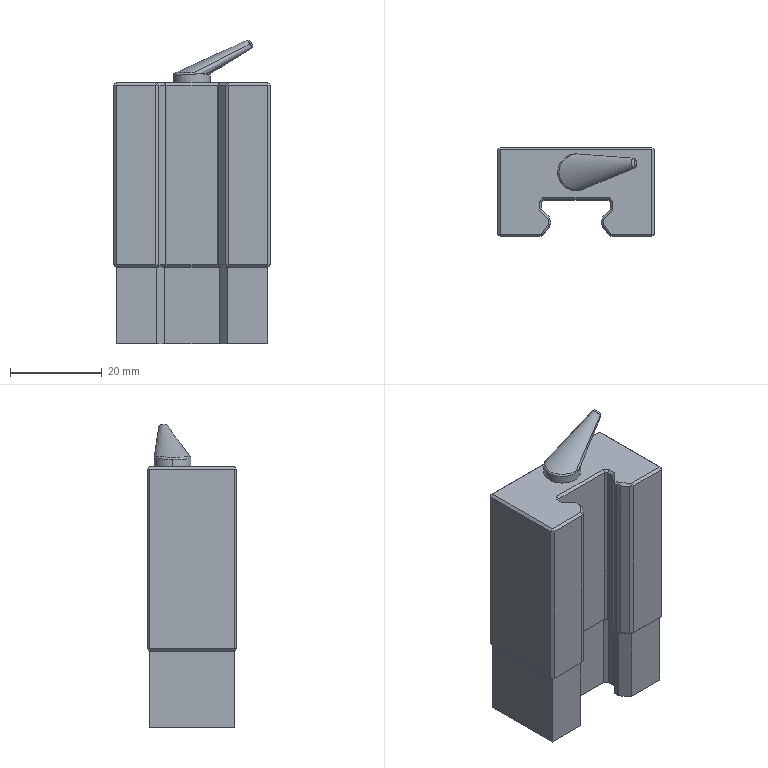Part | STEP file | SM140A-20-1140D-SM140F-140w-700EGH15SA | 1 solid | 145 faces | box 34 x 19.5 x 66.139 mm | volume 30467 mm3 | plane 85 | spline 42 | cylinder 14 | cone 4 | commonest cylinder face diameters 3.2 x8 3.3 x4 8 x2